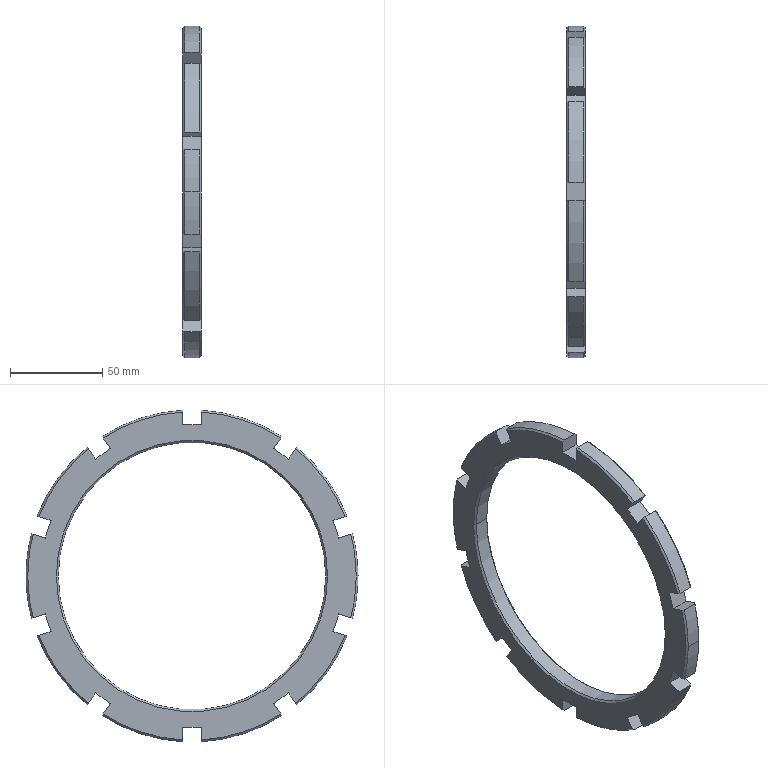Part | NX | features BREP 1 | 1 solid | 74 faces | box 10 x 180 x 179.722 mm | volume 80464 mm3 | plane 32 | cone 28 | cylinder 14 | commonest cylinder face diameters 180 x12 145 x2